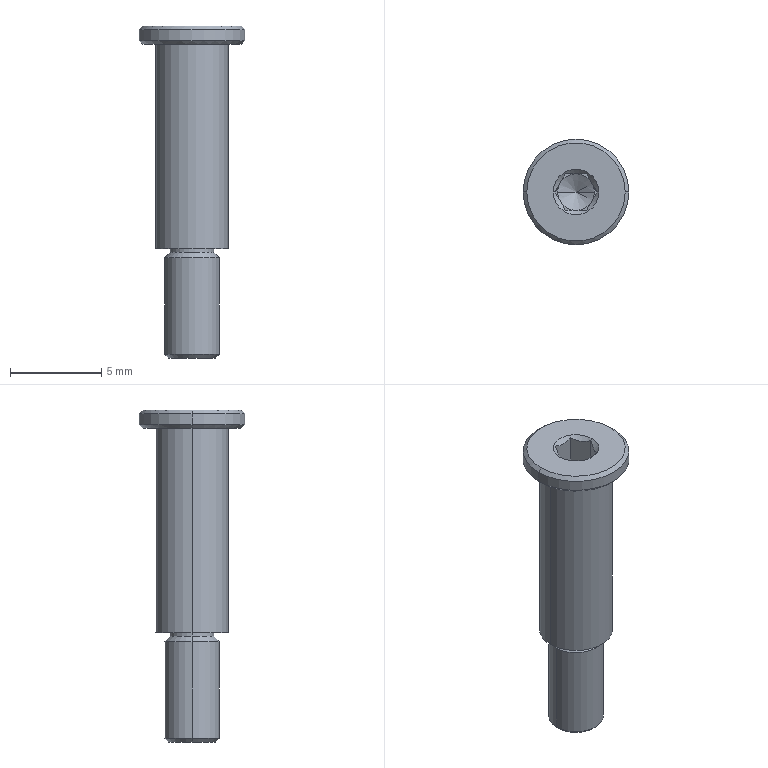Part | SolidWorks | features HoleWzd 1, ICE 1, Revolution 1 | 1 solid | 36 faces | box 5.8 x 5.8 x 18.2 mm | volume 198.341 mm3 | plane 16 | cone 12 | cylinder 8 | commonest cylinder face diameters 2.4 x2 3 x2 4 x2 5.8 x2
STEP:
#1=CARTESIAN_POINT('',(0.,0.,-3.101));
#2=VERTEX_POINT('',#1);
#3=CARTESIAN_POINT('',(1.,0.,-2.5));
#4=VERTEX_POINT('',#3);
#5=CARTESIAN_POINT('',(1.,0.,-2.5));
#6=DIRECTION('',(0.8572,0.,0.515));
#7=VECTOR('',#6,1000.);
#8=LINE('',#5,#7);
#9=EDGE_CURVE('',#2,#4,#8,.T.);
#10=ORIENTED_EDGE('',*,*,#9,.F.);
#11=CARTESIAN_POINT('',(-1.,0.,-2.5));
#12=VERTEX_POINT('',#11);
#13=CARTESIAN_POINT('',(-1.,0.,-2.5));
#14=DIRECTION('',(-0.8572,0.,0.515));
#15=VECTOR('',#14,1000.);
#16=LINE('',#13,#15);
#17=EDGE_CURVE('',#2,#12,#16,.T.);
#18=ORIENTED_EDGE('',*,*,#17,.T.);
#19=CARTESIAN_POINT('',(-0.866,-0.5,-2.5));
#20=VERTEX_POINT('',#19);
#21=CARTESIAN_POINT('',(0.,0.,-2.5));
#22=DIRECTION('',(0.,0.,1.));
#23=DIRECTION('',(1.,0.,0.));
#24=AXIS2_PLACEMENT_3D('',#21,#22,#23);
#25=CIRCLE('',#24,1.);
#26=EDGE_CURVE('',#12,#20,#25,.T.);
#27=ORIENTED_EDGE('',*,*,#26,.T.);
#28=CARTESIAN_POINT('',(0.,-1.,-2.5));
#29=VERTEX_POINT('',#28);
#30=CARTESIAN_POINT('',(0.,0.,-2.5));
#31=DIRECTION('',(0.,0.,1.));
#32=DIRECTION('',(1.,0.,0.));
#33=AXIS2_PLACEMENT_3D('',#30,#31,#32);
#34=CIRCLE('',#33,1.);
#35=EDGE_CURVE('',#20,#29,#34,.T.);
#36=ORIENTED_EDGE('',*,*,#35,.T.);
#37=CARTESIAN_POINT('',(0.866,-0.5,-2.5));
#38=VERTEX_POINT('',#37);
#39=CARTESIAN_POINT('',(0.,0.,-2.5));
#40=DIRECTION('',(0.,0.,1.));
#41=DIRECTION('',(1.,0.,0.));
#42=AXIS2_PLACEMENT_3D('',#39,#40,#41);
#43=CIRCLE('',#42,1.);
#44=EDGE_CURVE('',#29,#38,#43,.T.);
#45=ORIENTED_EDGE('',*,*,#44,.T.);
#46=CARTESIAN_POINT('',(0.,0.,-2.5));
#47=DIRECTION('',(0.,0.,1.));
#48=DIRECTION('',(1.,0.,0.));
#49=AXIS2_PLACEMENT_3D('',#46,#47,#48);
#50=CIRCLE('',#49,1.);
#51=EDGE_CURVE('',#38,#4,#50,.T.);
#52=ORIENTED_EDGE('',*,*,#51,.T.);
#53=EDGE_LOOP('',(#10,#18,#27,#36,#45,#52));
#54=FACE_OUTER_BOUND('',#53,.T.);
#55=CARTESIAN_POINT('',(0.,0.,-2.5));
#56=DIRECTION('',(0.,0.,1.));
#57=DIRECTION('',(1.,0.,0.));
#58=AXIS2_PLACEMENT_3D('',#55,#56,#57);
#59=CONICAL_SURFACE('',#58,1.,1.03);
#60=ADVANCED_FACE('',(#54),#59,.F.);
#61=CARTESIAN_POINT('',(-0.5774,-1.,-0.0953));
#62=VERTEX_POINT('',#61);
#63=CARTESIAN_POINT('',(-1.155,0.,-0.0953));
#64=VERTEX_POINT('',#63);
#65=CARTESIAN_POINT('',(-0.5774,-1.,-0.0953));
#66=CARTESIAN_POINT('',(-0.6225,-0.9219,-0.1404));
#67=CARTESIAN_POINT('',(-0.6686,-0.842,-0.1788));
#68=CARTESIAN_POINT('',(-0.7641,-0.6765,-0.2336));
#69=CARTESIAN_POINT('',(-0.8146,-0.5891,-0.2498));
#70=CARTESIAN_POINT('',(-0.9658,-0.3272,-0.2504));
#71=CARTESIAN_POINT('',(-1.064,-0.1572,-0.186));
#72=CARTESIAN_POINT('',(-1.155,0.,-0.0953));
#73=B_SPLINE_CURVE_WITH_KNOTS('',3,(#65,#66,#67,#68,#69,#70,#71,#72),.UNSPECIFIED.,.F.,.F.,(4,2,2,4),(0.000000254,0.0002984,0.0005966,0.001193),.UNSPECIFIED.);
#74=EDGE_CURVE('',#62,#64,#73,.T.);
#75=ORIENTED_EDGE('',*,*,#74,.T.);
#76=CARTESIAN_POINT('',(-1.25,0.,0.));
#77=VERTEX_POINT('',#76);
#78=CARTESIAN_POINT('',(-1.25,0.,0.));
#79=DIRECTION('',(-0.7071,0.,0.7071));
#80=VECTOR('',#79,1000.);
#81=LINE('',#78,#80);
#82=EDGE_CURVE('',#64,#77,#81,.T.);
#83=ORIENTED_EDGE('',*,*,#82,.T.);
#84=CARTESIAN_POINT('',(1.25,0.,0.));
#85=VERTEX_POINT('',#84);
#86=CARTESIAN_POINT('',(0.,0.,0.));
#87=DIRECTION('',(0.,0.,1.));
#88=DIRECTION('',(1.,0.,0.));
#89=AXIS2_PLACEMENT_3D('',#86,#87,#88);
#90=CIRCLE('',#89,1.25);
#91=EDGE_CURVE('',#77,#85,#90,.T.);
#92=ORIENTED_EDGE('',*,*,#91,.T.);
#93=CARTESIAN_POINT('',(1.155,0.,-0.0953));
#94=VERTEX_POINT('',#93);
#95=CARTESIAN_POINT('',(1.25,0.,0.));
#96=DIRECTION('',(0.7071,0.,0.7071));
#97=VECTOR('',#96,1000.);
#98=LINE('',#95,#97);
#99=EDGE_CURVE('',#94,#85,#98,.T.);
#100=ORIENTED_EDGE('',*,*,#99,.F.);
#101=CARTESIAN_POINT('',(0.5774,-1.,-0.0953));
#102=VERTEX_POINT('',#101);
#103=CARTESIAN_POINT('',(1.155,0.,-0.0953));
#104=CARTESIAN_POINT('',(1.11,-0.07813,-0.1404));
#105=CARTESIAN_POINT('',(1.063,-0.158,-0.1788));
#106=CARTESIAN_POINT('',(0.9679,-0.3235,-0.2336));
#107=CARTESIAN_POINT('',(0.9175,-0.4109,-0.2498));
#108=CARTESIAN_POINT('',(0.7663,-0.6728,-0.2504));
#109=CARTESIAN_POINT('',(0.6681,-0.8428,-0.186));
#110=CARTESIAN_POINT('',(0.5774,-1.,-0.0953));
#111=B_SPLINE_CURVE_WITH_KNOTS('',3,(#103,#104,#105,#106,#107,#108,#109,#110),.UNSPECIFIED.,.F.,.F.,(4,2,2,4),(0.000000254,0.0002984,0.0005966,0.001193),.UNSPECIFIED.);
#112=EDGE_CURVE('',#94,#102,#111,.T.);
#113=ORIENTED_EDGE('',*,*,#112,.T.);
#114=CARTESIAN_POINT('',(0.5774,-1.,-0.0953));
#115=CARTESIAN_POINT('',(0.3985,-1.,-0.1847));
#116=CARTESIAN_POINT('',(0.2033,-1.,-0.2499));
#117=CARTESIAN_POINT('',(-0.2019,-1.,-0.2501));
#118=CARTESIAN_POINT('',(-0.398,-1.,-0.185));
#119=CARTESIAN_POINT('',(-0.5774,-1.,-0.0953));
#120=B_SPLINE_CURVE_WITH_KNOTS('',3,(#114,#115,#116,#117,#118,#119),.UNSPECIFIED.,.F.,.F.,(4,2,4),(0.001472,0.002073,0.002675),.UNSPECIFIED.);
#121=EDGE_CURVE('',#102,#62,#120,.T.);
#122=ORIENTED_EDGE('',*,*,#121,.T.);
#123=EDGE_LOOP('',(#75,#83,#92,#100,#113,#122));
#124=FACE_OUTER_BOUND('',#123,.T.);
#125=CARTESIAN_POINT('',(0.,0.,0.));
#126=DIRECTION('',(0.,0.,1.));
#127=DIRECTION('',(1.,0.,0.));
#128=AXIS2_PLACEMENT_3D('',#125,#126,#127);
#129=CONICAL_SURFACE('',#128,1.25,0.7854);
#130=ADVANCED_FACE('',(#124),#129,.F.);
#131=CARTESIAN_POINT('',(1.3,0.,-18.2));
#132=VERTEX_POINT('',#131);
#133=CARTESIAN_POINT('',(-1.3,0.,-18.2));
#134=VERTEX_POINT('',#133);
#135=CARTESIAN_POINT('',(0.,0.,-18.2));
#136=DIRECTION('',(0.,0.,1.));
#137=DIRECTION('',(1.,0.,0.));
#138=AXIS2_PLACEMENT_3D('',#135,#136,#137);
#139=CIRCLE('',#138,1.3);
#140=EDGE_CURVE('',#132,#134,#139,.T.);
#141=ORIENTED_EDGE('',*,*,#140,.T.);
#142=CARTESIAN_POINT('',(-1.5,0.,-18.));
#143=VERTEX_POINT('',#142);
#144=CARTESIAN_POINT('',(-1.5,0.,-18.));
#145=DIRECTION('',(-0.7071,0.,0.7071));
#146=VECTOR('',#145,1000.);
#147=LINE('',#144,#146);
#148=EDGE_CURVE('',#134,#143,#147,.T.);
#149=ORIENTED_EDGE('',*,*,#148,.T.);
#150=CARTESIAN_POINT('',(1.5,0.,-18.));
#151=VERTEX_POINT('',#150);
#152=CARTESIAN_POINT('',(0.,0.,-18.));
#153=DIRECTION('',(0.,0.,1.));
#154=DIRECTION('',(1.,0.,0.));
#155=AXIS2_PLACEMENT_3D('',#152,#153,#154);
#156=CIRCLE('',#155,1.5);
#157=EDGE_CURVE('',#151,#143,#156,.T.);
#158=ORIENTED_EDGE('',*,*,#157,.F.);
#159=CARTESIAN_POINT('',(1.5,0.,-18.));
#160=DIRECTION('',(0.7071,0.,0.7071));
#161=VECTOR('',#160,1000.);
#162=LINE('',#159,#161);
#163=EDGE_CURVE('',#132,#151,#162,.T.);
#164=ORIENTED_EDGE('',*,*,#163,.F.);
#165=EDGE_LOOP('',(#141,#149,#158,#164));
#166=FACE_OUTER_BOUND('',#165,.T.);
#167=CARTESIAN_POINT('',(0.,0.,-18.));
#168=DIRECTION('',(0.,0.,1.));
#169=DIRECTION('',(1.,0.,0.));
#170=AXIS2_PLACEMENT_3D('',#167,#168,#169);
#171=CONICAL_SURFACE('',#170,1.5,0.7854);
#172=ADVANCED_FACE('',(#166),#171,.T.);
#173=ORIENTED_EDGE('',*,*,#157,.T.);
#174=CARTESIAN_POINT('',(-1.5,0.,-12.7));
#175=VERTEX_POINT('',#174);
#176=CARTESIAN_POINT('',(-1.5,0.,4.426));
#177=DIRECTION('',(0.,0.,1.));
#178=VECTOR('',#177,1000.);
#179=LINE('',#176,#178);
#180=EDGE_CURVE('',#143,#175,#179,.T.);
#181=ORIENTED_EDGE('',*,*,#180,.T.);
#182=CARTESIAN_POINT('',(1.5,0.,-12.7));
#183=VERTEX_POINT('',#182);
#184=CARTESIAN_POINT('',(0.,0.,-12.7));
#185=DIRECTION('',(0.,0.,1.));
#186=DIRECTION('',(1.,0.,0.));
#187=AXIS2_PLACEMENT_3D('',#184,#185,#186);
#188=CIRCLE('',#187,1.5);
#189=EDGE_CURVE('',#183,#175,#188,.T.);
#190=ORIENTED_EDGE('',*,*,#189,.F.);
#191=CARTESIAN_POINT('',(1.5,0.,4.426));
#192=DIRECTION('',(0.,0.,1.));
#193=VECTOR('',#192,1000.);
#194=LINE('',#191,#193);
#195=EDGE_CURVE('',#151,#183,#194,.T.);
#196=ORIENTED_EDGE('',*,*,#195,.F.);
#197=EDGE_LOOP('',(#173,#181,#190,#196));
#198=FACE_OUTER_BOUND('',#197,.T.);
#199=CARTESIAN_POINT('',(0.,0.,4.426));
#200=DIRECTION('',(0.,0.,1.));
#201=DIRECTION('',(1.,0.,0.));
#202=AXIS2_PLACEMENT_3D('',#199,#200,#201);
#203=CYLINDRICAL_SURFACE('',#202,1.5);
#204=ADVANCED_FACE('',(#198),#203,.T.);
#205=CARTESIAN_POINT('',(1.2,0.,-12.4));
#206=VERTEX_POINT('',#205);
#207=CARTESIAN_POINT('',(-1.2,0.,-12.4));
#208=VERTEX_POINT('',#207);
#209=CARTESIAN_POINT('',(0.,0.,-12.4));
#210=DIRECTION('',(0.,0.,1.));
#211=DIRECTION('',(1.,0.,0.));
#212=AXIS2_PLACEMENT_3D('',#209,#210,#211);
#213=CIRCLE('',#212,1.2);
#214=EDGE_CURVE('',#206,#208,#213,.T.);
#215=ORIENTED_EDGE('',*,*,#214,.F.);
#216=CARTESIAN_POINT('',(1.2,0.,-12.4));
#217=DIRECTION('',(0.7071,0.,-0.7071));
#218=VECTOR('',#217,1000.);
#219=LINE('',#216,#218);
#220=EDGE_CURVE('',#206,#183,#219,.T.);
#221=ORIENTED_EDGE('',*,*,#220,.T.);
#222=ORIENTED_EDGE('',*,*,#189,.T.);
#223=CARTESIAN_POINT('',(-1.2,0.,-12.4));
#224=DIRECTION('',(-0.7071,0.,-0.7071));
#225=VECTOR('',#224,1000.);
#226=LINE('',#223,#225);
#227=EDGE_CURVE('',#208,#175,#226,.T.);
#228=ORIENTED_EDGE('',*,*,#227,.F.);
#229=EDGE_LOOP('',(#215,#221,#222,#228));
#230=FACE_OUTER_BOUND('',#229,.T.);
#231=CARTESIAN_POINT('',(0.,0.,-12.4));
#232=DIRECTION('',(0.,0.,-1.));
#233=DIRECTION('',(-1.,0.,0.));
#234=AXIS2_PLACEMENT_3D('',#231,#232,#233);
#235=CONICAL_SURFACE('',#234,1.2,0.7854);
#236=ADVANCED_FACE('',(#230),#235,.T.);
#237=ORIENTED_EDGE('',*,*,#214,.T.);
#238=CARTESIAN_POINT('',(-1.2,0.,-12.2));
#239=VERTEX_POINT('',#238);
#240=CARTESIAN_POINT('',(-1.2,0.,4.426));
#241=DIRECTION('',(0.,0.,1.));
#242=VECTOR('',#241,1000.);
#243=LINE('',#240,#242);
#244=EDGE_CURVE('',#208,#239,#243,.T.);
#245=ORIENTED_EDGE('',*,*,#244,.T.);
#246=CARTESIAN_POINT('',(1.2,0.,-12.2));
#247=VERTEX_POINT('',#246);
#248=CARTESIAN_POINT('',(0.,0.,-12.2));
#249=DIRECTION('',(0.,0.,1.));
#250=DIRECTION('',(1.,0.,0.));
#251=AXIS2_PLACEMENT_3D('',#248,#249,#250);
#252=CIRCLE('',#251,1.2);
#253=EDGE_CURVE('',#247,#239,#252,.T.);
#254=ORIENTED_EDGE('',*,*,#253,.F.);
#255=CARTESIAN_POINT('',(1.2,0.,4.426));
#256=DIRECTION('',(0.,0.,1.));
#257=VECTOR('',#256,1000.);
#258=LINE('',#255,#257);
#259=EDGE_CURVE('',#206,#247,#258,.T.);
#260=ORIENTED_EDGE('',*,*,#259,.F.);
#261=EDGE_LOOP('',(#237,#245,#254,#260));
#262=FACE_OUTER_BOUND('',#261,.T.);
#263=CARTESIAN_POINT('',(0.,0.,4.426));
#264=DIRECTION('',(0.,0.,1.));
#265=DIRECTION('',(1.,0.,0.));
#266=AXIS2_PLACEMENT_3D('',#263,#264,#265);
#267=CYLINDRICAL_SURFACE('',#266,1.2);
#268=ADVANCED_FACE('',(#262),#267,.T.);
#269=CARTESIAN_POINT('',(2.,0.,-12.2));
#270=VERTEX_POINT('',#269);
#271=CARTESIAN_POINT('',(-2.,0.,-12.2));
#272=VERTEX_POINT('',#271);
#273=CARTESIAN_POINT('',(0.,0.,-12.2));
#274=DIRECTION('',(0.,0.,1.));
#275=DIRECTION('',(1.,0.,0.));
#276=AXIS2_PLACEMENT_3D('',#273,#274,#275);
#277=CIRCLE('',#276,2.);
#278=EDGE_CURVE('',#270,#272,#277,.T.);
#279=ORIENTED_EDGE('',*,*,#278,.T.);
#280=CARTESIAN_POINT('',(-2.,0.,-1.));
#281=VERTEX_POINT('',#280);
#282=CARTESIAN_POINT('',(-2.,0.,4.426));
#283=DIRECTION('',(0.,0.,1.));
#284=VECTOR('',#283,1000.);
#285=LINE('',#282,#284);
#286=EDGE_CURVE('',#272,#281,#285,.T.);
#287=ORIENTED_EDGE('',*,*,#286,.T.);
#288=CARTESIAN_POINT('',(2.,0.,-1.));
#289=VERTEX_POINT('',#288);
#290=CARTESIAN_POINT('',(0.,0.,-1.));
#291=DIRECTION('',(0.,0.,1.));
#292=DIRECTION('',(1.,0.,0.));
#293=AXIS2_PLACEMENT_3D('',#290,#291,#292);
#294=CIRCLE('',#293,2.);
#295=EDGE_CURVE('',#289,#281,#294,.T.);
#296=ORIENTED_EDGE('',*,*,#295,.F.);
#297=CARTESIAN_POINT('',(2.,0.,4.426));
#298=DIRECTION('',(0.,0.,1.));
#299=VECTOR('',#298,1000.);
#300=LINE('',#297,#299);
#301=EDGE_CURVE('',#270,#289,#300,.T.);
#302=ORIENTED_EDGE('',*,*,#301,.F.);
#303=EDGE_LOOP('',(#279,#287,#296,#302));
#304=FACE_OUTER_BOUND('',#303,.T.);
#305=CARTESIAN_POINT('',(0.,0.,4.426));
#306=DIRECTION('',(0.,0.,1.));
#307=DIRECTION('',(1.,0.,0.));
#308=AXIS2_PLACEMENT_3D('',#305,#306,#307);
#309=CYLINDRICAL_SURFACE('',#308,2.);
#310=ADVANCED_FACE('',(#304),#309,.T.);
#311=CARTESIAN_POINT('',(2.7,0.,-1.));
#312=VERTEX_POINT('',#311);
#313=CARTESIAN_POINT('',(-2.7,0.,-1.));
#314=VERTEX_POINT('',#313);
#315=CARTESIAN_POINT('',(0.,0.,-1.));
#316=DIRECTION('',(0.,0.,1.));
#317=DIRECTION('',(1.,0.,0.));
#318=AXIS2_PLACEMENT_3D('',#315,#316,#317);
#319=CIRCLE('',#318,2.7);
#320=EDGE_CURVE('',#312,#314,#319,.T.);
#321=ORIENTED_EDGE('',*,*,#320,.T.);
#322=CARTESIAN_POINT('',(-2.9,0.,-0.8));
#323=VERTEX_POINT('',#322);
#324=CARTESIAN_POINT('',(-2.9,0.,-0.8));
#325=DIRECTION('',(-0.7071,0.,0.7071));
#326=VECTOR('',#325,1000.);
#327=LINE('',#324,#326);
#328=EDGE_CURVE('',#314,#323,#327,.T.);
#329=ORIENTED_EDGE('',*,*,#328,.T.);
#330=CARTESIAN_POINT('',(2.9,0.,-0.8));
#331=VERTEX_POINT('',#330);
#332=CARTESIAN_POINT('',(0.,0.,-0.8));
#333=DIRECTION('',(0.,0.,1.));
#334=DIRECTION('',(1.,0.,0.));
#335=AXIS2_PLACEMENT_3D('',#332,#333,#334);
#336=CIRCLE('',#335,2.9);
#337=EDGE_CURVE('',#331,#323,#336,.T.);
#338=ORIENTED_EDGE('',*,*,#337,.F.);
#339=CARTESIAN_POINT('',(2.9,0.,-0.8));
#340=DIRECTION('',(0.7071,0.,0.7071));
#341=VECTOR('',#340,1000.);
#342=LINE('',#339,#341);
#343=EDGE_CURVE('',#312,#331,#342,.T.);
#344=ORIENTED_EDGE('',*,*,#343,.F.);
#345=EDGE_LOOP('',(#321,#329,#338,#344));
#346=FACE_OUTER_BOUND('',#345,.T.);
#347=CARTESIAN_POINT('',(0.,0.,-0.8));
#348=DIRECTION('',(0.,0.,1.));
#349=DIRECTION('',(1.,0.,0.));
#350=AXIS2_PLACEMENT_3D('',#347,#348,#349);
#351=CONICAL_SURFACE('',#350,2.9,0.7854);
#352=ADVANCED_FACE('',(#346),#351,.T.);
#353=ORIENTED_EDGE('',*,*,#337,.T.);
#354=CARTESIAN_POINT('',(-2.9,0.,-0.2));
#355=VERTEX_POINT('',#354);
#356=CARTESIAN_POINT('',(-2.9,0.,4.426));
#357=DIRECTION('',(0.,0.,1.));
#358=VECTOR('',#357,1000.);
#359=LINE('',#356,#358);
#360=EDGE_CURVE('',#323,#355,#359,.T.);
#361=ORIENTED_EDGE('',*,*,#360,.T.);
#362=CARTESIAN_POINT('',(2.9,0.,-0.2));
#363=VERTEX_POINT('',#362);
#364=CARTESIAN_POINT('',(0.,0.,-0.2));
#365=DIRECTION('',(0.,0.,1.));
#366=DIRECTION('',(1.,0.,0.));
#367=AXIS2_PLACEMENT_3D('',#364,#365,#366);
#368=CIRCLE('',#367,2.9);
#369=EDGE_CURVE('',#363,#355,#368,.T.);
#370=ORIENTED_EDGE('',*,*,#369,.F.);
#371=CARTESIAN_POINT('',(2.9,0.,4.426));
#372=DIRECTION('',(0.,0.,1.));
#373=VECTOR('',#372,1000.);
#374=LINE('',#371,#373);
#375=EDGE_CURVE('',#331,#363,#374,.T.);
#376=ORIENTED_EDGE('',*,*,#375,.F.);
#377=EDGE_LOOP('',(#353,#361,#370,#376));
#378=FACE_OUTER_BOUND('',#377,.T.);
#379=CARTESIAN_POINT('',(0.,0.,4.426));
#380=DIRECTION('',(0.,0.,1.));
#381=DIRECTION('',(1.,0.,0.));
#382=AXIS2_PLACEMENT_3D('',#379,#380,#381);
#383=CYLINDRICAL_SURFACE('',#382,2.9);
#384=ADVANCED_FACE('',(#378),#383,.T.);
#385=CARTESIAN_POINT('',(2.7,0.,0.));
#386=VERTEX_POINT('',#385);
#387=CARTESIAN_POINT('',(-2.7,0.,0.));
#388=VERTEX_POINT('',#387);
#389=CARTESIAN_POINT('',(0.,0.,0.));
#390=DIRECTION('',(0.,0.,1.));
#391=DIRECTION('',(1.,0.,0.));
#392=AXIS2_PLACEMENT_3D('',#389,#390,#391);
#393=CIRCLE('',#392,2.7);
#394=EDGE_CURVE('',#386,#388,#393,.T.);
#395=ORIENTED_EDGE('',*,*,#394,.F.);
#396=CARTESIAN_POINT('',(2.7,0.,0.));
#397=DIRECTION('',(0.7071,0.,-0.7071));
#398=VECTOR('',#397,1000.);
#399=LINE('',#396,#398);
#400=EDGE_CURVE('',#386,#363,#399,.T.);
#401=ORIENTED_EDGE('',*,*,#400,.T.);
#402=ORIENTED_EDGE('',*,*,#369,.T.);
#403=CARTESIAN_POINT('',(-2.7,0.,0.));
#404=DIRECTION('',(-0.7071,0.,-0.7071));
#405=VECTOR('',#404,1000.);
#406=LINE('',#403,#405);
#407=EDGE_CURVE('',#388,#355,#406,.T.);
#408=ORIENTED_EDGE('',*,*,#407,.F.);
#409=EDGE_LOOP('',(#395,#401,#402,#408));
#410=FACE_OUTER_BOUND('',#409,.T.);
#411=CARTESIAN_POINT('',(0.,0.,0.));
#412=DIRECTION('',(0.,0.,-1.));
#413=DIRECTION('',(-1.,0.,0.));
#414=AXIS2_PLACEMENT_3D('',#411,#412,#413);
#415=CONICAL_SURFACE('',#414,2.7,0.7854);
#416=ADVANCED_FACE('',(#410),#415,.T.);
#417=CARTESIAN_POINT('',(0.,0.,0.));
#418=DIRECTION('',(0.,0.,1.));
#419=DIRECTION('',(1.,0.,0.));
#420=AXIS2_PLACEMENT_3D('',#417,#418,#419);
#421=CIRCLE('',#420,1.25);
#422=EDGE_CURVE('',#85,#77,#421,.T.);
#423=ORIENTED_EDGE('',*,*,#422,.F.);
#424=ORIENTED_EDGE('',*,*,#91,.F.);
#425=EDGE_LOOP('',(#423,#424));
#426=FACE_BOUND('',#425,.T.);
#427=CARTESIAN_POINT('',(0.,0.,0.));
#428=DIRECTION('',(0.,0.,1.));
#429=DIRECTION('',(1.,0.,0.));
#430=AXIS2_PLACEMENT_3D('',#427,#428,#429);
#431=CIRCLE('',#430,2.7);
#432=EDGE_CURVE('',#388,#386,#431,.T.);
#433=ORIENTED_EDGE('',*,*,#432,.T.);
#434=ORIENTED_EDGE('',*,*,#394,.T.);
#435=EDGE_LOOP('',(#433,#434));
#436=FACE_OUTER_BOUND('',#435,.T.);
#437=CARTESIAN_POINT('',(0.,0.,0.));
#438=DIRECTION('',(0.,0.,1.));
#439=DIRECTION('',(1.,0.,0.));
#440=AXIS2_PLACEMENT_3D('',#437,#438,#439);
#441=PLANE('',#440);
#442=ADVANCED_FACE('',(#426,#436),#441,.T.);
#443=ORIENTED_EDGE('',*,*,#400,.F.);
#444=ORIENTED_EDGE('',*,*,#432,.F.);
#445=ORIENTED_EDGE('',*,*,#407,.T.);
#446=CARTESIAN_POINT('',(0.,0.,-0.2));
#447=DIRECTION('',(0.,0.,1.));
#448=DIRECTION('',(1.,0.,0.));
#449=AXIS2_PLACEMENT_3D('',#446,#447,#448);
#450=CIRCLE('',#449,2.9);
#451=EDGE_CURVE('',#355,#363,#450,.T.);
#452=ORIENTED_EDGE('',*,*,#451,.T.);
#453=EDGE_LOOP('',(#443,#444,#445,#452));
#454=FACE_OUTER_BOUND('',#453,.T.);
#455=CARTESIAN_POINT('',(0.,0.,0.));
#456=DIRECTION('',(0.,0.,-1.));
#457=DIRECTION('',(-1.,0.,0.));
#458=AXIS2_PLACEMENT_3D('',#455,#456,#457);
#459=CONICAL_SURFACE('',#458,2.7,0.7854);
#460=ADVANCED_FACE('',(#454),#459,.T.);
#461=ORIENTED_EDGE('',*,*,#360,.F.);
#462=CARTESIAN_POINT('',(0.,0.,-0.8));
#463=DIRECTION('',(0.,0.,1.));
#464=DIRECTION('',(1.,0.,0.));
#465=AXIS2_PLACEMENT_3D('',#462,#463,#464);
#466=CIRCLE('',#465,2.9);
#467=EDGE_CURVE('',#323,#331,#466,.T.);
#468=ORIENTED_EDGE('',*,*,#467,.T.);
#469=ORIENTED_EDGE('',*,*,#375,.T.);
#470=ORIENTED_EDGE('',*,*,#451,.F.);
#471=EDGE_LOOP('',(#461,#468,#469,#470));
#472=FACE_OUTER_BOUND('',#471,.T.);
#473=CARTESIAN_POINT('',(0.,0.,4.426));
#474=DIRECTION('',(0.,0.,1.));
#475=DIRECTION('',(1.,0.,0.));
#476=AXIS2_PLACEMENT_3D('',#473,#474,#475);
#477=CYLINDRICAL_SURFACE('',#476,2.9);
#478=ADVANCED_FACE('',(#472),#477,.T.);
#479=ORIENTED_EDGE('',*,*,#328,.F.);
#480=CARTESIAN_POINT('',(0.,0.,-1.));
#481=DIRECTION('',(0.,0.,1.));
#482=DIRECTION('',(1.,0.,0.));
#483=AXIS2_PLACEMENT_3D('',#480,#481,#482);
#484=CIRCLE('',#483,2.7);
#485=EDGE_CURVE('',#314,#312,#484,.T.);
#486=ORIENTED_EDGE('',*,*,#485,.T.);
#487=ORIENTED_EDGE('',*,*,#343,.T.);
#488=ORIENTED_EDGE('',*,*,#467,.F.);
#489=EDGE_LOOP('',(#479,#486,#487,#488));
#490=FACE_OUTER_BOUND('',#489,.T.);
#491=CARTESIAN_POINT('',(0.,0.,-0.8));
#492=DIRECTION('',(0.,0.,1.));
#493=DIRECTION('',(1.,0.,0.));
#494=AXIS2_PLACEMENT_3D('',#491,#492,#493);
#495=CONICAL_SURFACE('',#494,2.9,0.7854);
#496=ADVANCED_FACE('',(#490),#495,.T.);
#497=ORIENTED_EDGE('',*,*,#295,.T.);
#498=CARTESIAN_POINT('',(0.,0.,-1.));
#499=DIRECTION('',(0.,0.,1.));
#500=DIRECTION('',(1.,0.,0.));
#501=AXIS2_PLACEMENT_3D('',#498,#499,#500);
#502=CIRCLE('',#501,2.);
#503=EDGE_CURVE('',#281,#289,#502,.T.);
#504=ORIENTED_EDGE('',*,*,#503,.T.);
#505=EDGE_LOOP('',(#497,#504));
#506=FACE_BOUND('',#505,.T.);
#507=ORIENTED_EDGE('',*,*,#320,.F.);
#508=ORIENTED_EDGE('',*,*,#485,.F.);
#509=EDGE_LOOP('',(#507,#508));
#510=FACE_OUTER_BOUND('',#509,.T.);
#511=CARTESIAN_POINT('',(2.7,0.,-1.));
#512=DIRECTION('',(0.,0.,-1.));
#513=DIRECTION('',(-1.,0.,0.));
#514=AXIS2_PLACEMENT_3D('',#511,#512,#513);
#515=PLANE('',#514);
#516=ADVANCED_FACE('',(#506,#510),#515,.T.);
#517=ORIENTED_EDGE('',*,*,#286,.F.);
#518=CARTESIAN_POINT('',(0.,0.,-12.2));
#519=DIRECTION('',(0.,0.,1.));
#520=DIRECTION('',(1.,0.,0.));
#521=AXIS2_PLACEMENT_3D('',#518,#519,#520);
#522=CIRCLE('',#521,2.);
#523=EDGE_CURVE('',#272,#270,#522,.T.);
#524=ORIENTED_EDGE('',*,*,#523,.T.);
#525=ORIENTED_EDGE('',*,*,#301,.T.);
#526=ORIENTED_EDGE('',*,*,#503,.F.);
#527=EDGE_LOOP('',(#517,#524,#525,#526));
#528=FACE_OUTER_BOUND('',#527,.T.);
#529=CARTESIAN_POINT('',(0.,0.,4.426));
#530=DIRECTION('',(0.,0.,1.));
#531=DIRECTION('',(1.,0.,0.));
#532=AXIS2_PLACEMENT_3D('',#529,#530,#531);
#533=CYLINDRICAL_SURFACE('',#532,2.);
#534=ADVANCED_FACE('',(#528),#533,.T.);
#535=ORIENTED_EDGE('',*,*,#253,.T.);
#536=CARTESIAN_POINT('',(0.,0.,-12.2));
#537=DIRECTION('',(0.,0.,1.));
#538=DIRECTION('',(1.,0.,0.));
#539=AXIS2_PLACEMENT_3D('',#536,#537,#538);
#540=CIRCLE('',#539,1.2);
#541=EDGE_CURVE('',#239,#247,#540,.T.);
#542=ORIENTED_EDGE('',*,*,#541,.T.);
#543=EDGE_LOOP('',(#535,#542));
#544=FACE_BOUND('',#543,.T.);
#545=ORIENTED_EDGE('',*,*,#278,.F.);
#546=ORIENTED_EDGE('',*,*,#523,.F.);
#547=EDGE_LOOP('',(#545,#546));
#548=FACE_OUTER_BOUND('',#547,.T.);
#549=CARTESIAN_POINT('',(2.,0.,-12.2));
#550=DIRECTION('',(0.,0.,-1.));
#551=DIRECTION('',(-1.,0.,0.));
#552=AXIS2_PLACEMENT_3D('',#549,#550,#551);
#553=PLANE('',#552);
#554=ADVANCED_FACE('',(#544,#548),#553,.T.);
#555=ORIENTED_EDGE('',*,*,#244,.F.);
#556=CARTESIAN_POINT('',(0.,0.,-12.4));
#557=DIRECTION('',(0.,0.,1.));
#558=DIRECTION('',(1.,0.,0.));
#559=AXIS2_PLACEMENT_3D('',#556,#557,#558);
#560=CIRCLE('',#559,1.2);
#561=EDGE_CURVE('',#208,#206,#560,.T.);
#562=ORIENTED_EDGE('',*,*,#561,.T.);
#563=ORIENTED_EDGE('',*,*,#259,.T.);
#564=ORIENTED_EDGE('',*,*,#541,.F.);
#565=EDGE_LOOP('',(#555,#562,#563,#564));
#566=FACE_OUTER_BOUND('',#565,.T.);
#567=CARTESIAN_POINT('',(0.,0.,4.426));
#568=DIRECTION('',(0.,0.,1.));
#569=DIRECTION('',(1.,0.,0.));
#570=AXIS2_PLACEMENT_3D('',#567,#568,#569);
#571=CYLINDRICAL_SURFACE('',#570,1.2);
#572=ADVANCED_FACE('',(#566),#571,.T.);
#573=ORIENTED_EDGE('',*,*,#220,.F.);
#574=ORIENTED_EDGE('',*,*,#561,.F.);
#575=ORIENTED_EDGE('',*,*,#227,.T.);
#576=CARTESIAN_POINT('',(0.,0.,-12.7));
#577=DIRECTION('',(0.,0.,1.));
#578=DIRECTION('',(1.,0.,0.));
#579=AXIS2_PLACEMENT_3D('',#576,#577,#578);
#580=CIRCLE('',#579,1.5);
#581=EDGE_CURVE('',#175,#183,#580,.T.);
#582=ORIENTED_EDGE('',*,*,#581,.T.);
#583=EDGE_LOOP('',(#573,#574,#575,#582));
#584=FACE_OUTER_BOUND('',#583,.T.);
#585=CARTESIAN_POINT('',(0.,0.,-12.4));
#586=DIRECTION('',(0.,0.,-1.));
#587=DIRECTION('',(-1.,0.,0.));
#588=AXIS2_PLACEMENT_3D('',#585,#586,#587);
#589=CONICAL_SURFACE('',#588,1.2,0.7854);
#590=ADVANCED_FACE('',(#584),#589,.T.);
#591=ORIENTED_EDGE('',*,*,#180,.F.);
#592=CARTESIAN_POINT('',(0.,0.,-18.));
#593=DIRECTION('',(0.,0.,1.));
#594=DIRECTION('',(1.,0.,0.));
#595=AXIS2_PLACEMENT_3D('',#592,#593,#594);
#596=CIRCLE('',#595,1.5);
#597=EDGE_CURVE('',#143,#151,#596,.T.);
#598=ORIENTED_EDGE('',*,*,#597,.T.);
#599=ORIENTED_EDGE('',*,*,#195,.T.);
#600=ORIENTED_EDGE('',*,*,#581,.F.);
#601=EDGE_LOOP('',(#591,#598,#599,#600));
#602=FACE_OUTER_BOUND('',#601,.T.);
#603=CARTESIAN_POINT('',(0.,0.,4.426));
#604=DIRECTION('',(0.,0.,1.));
#605=DIRECTION('',(1.,0.,0.));
#606=AXIS2_PLACEMENT_3D('',#603,#604,#605);
#607=CYLINDRICAL_SURFACE('',#606,1.5);
#608=ADVANCED_FACE('',(#602),#607,.T.);
#609=ORIENTED_EDGE('',*,*,#148,.F.);
#610=CARTESIAN_POINT('',(0.,0.,-18.2));
#611=DIRECTION('',(0.,0.,1.));
#612=DIRECTION('',(1.,0.,0.));
#613=AXIS2_PLACEMENT_3D('',#610,#611,#612);
#614=CIRCLE('',#613,1.3);
#615=EDGE_CURVE('',#134,#132,#614,.T.);
#616=ORIENTED_EDGE('',*,*,#615,.T.);
#617=ORIENTED_EDGE('',*,*,#163,.T.);
#618=ORIENTED_EDGE('',*,*,#597,.F.);
#619=EDGE_LOOP('',(#609,#616,#617,#618));
#620=FACE_OUTER_BOUND('',#619,.T.);
#621=CARTESIAN_POINT('',(0.,0.,-18.));
#622=DIRECTION('',(0.,0.,1.));
#623=DIRECTION('',(1.,0.,0.));
#624=AXIS2_PLACEMENT_3D('',#621,#622,#623);
#625=CONICAL_SURFACE('',#624,1.5,0.7854);
#626=ADVANCED_FACE('',(#620),#625,.T.);
#627=ORIENTED_EDGE('',*,*,#140,.F.);
#628=ORIENTED_EDGE('',*,*,#615,.F.);
#629=EDGE_LOOP('',(#627,#628));
#630=FACE_OUTER_BOUND('',#629,.T.);
#631=CARTESIAN_POINT('',(1.3,0.,-18.2));
#632=DIRECTION('',(0.,0.,-1.));
#633=DIRECTION('',(-1.,0.,0.));
#634=AXIS2_PLACEMENT_3D('',#631,#632,#633);
#635=PLANE('',#634);
#636=ADVANCED_FACE('',(#630),#635,.T.);
#637=ORIENTED_EDGE('',*,*,#82,.F.);
#638=CARTESIAN_POINT('',(-0.5774,1.,-0.0953));
#639=VERTEX_POINT('',#638);
#640=CARTESIAN_POINT('',(-1.155,0.,-0.0953));
#641=CARTESIAN_POINT('',(-1.11,0.07813,-0.1404));
#642=CARTESIAN_POINT('',(-1.063,0.158,-0.1788));
#643=CARTESIAN_POINT('',(-0.9679,0.3235,-0.2336));
#644=CARTESIAN_POINT('',(-0.9175,0.4109,-0.2498));
#645=CARTESIAN_POINT('',(-0.7663,0.6728,-0.2504));
#646=CARTESIAN_POINT('',(-0.6681,0.8428,-0.186));
#647=CARTESIAN_POINT('',(-0.5774,1.,-0.0953));
#648=B_SPLINE_CURVE_WITH_KNOTS('',3,(#640,#641,#642,#643,#644,#645,#646,#647),.UNSPECIFIED.,.F.,.F.,(4,2,2,4),(0.000000254,0.0002984,0.0005966,0.001193),.UNSPECIFIED.);
#649=EDGE_CURVE('',#64,#639,#648,.T.);
#650=ORIENTED_EDGE('',*,*,#649,.T.);
#651=CARTESIAN_POINT('',(0.5774,1.,-0.0953));
#652=VERTEX_POINT('',#651);
#653=CARTESIAN_POINT('',(-0.5774,1.,-0.0953));
#654=CARTESIAN_POINT('',(-0.3985,1.,-0.1847));
#655=CARTESIAN_POINT('',(-0.2033,1.,-0.2499));
#656=CARTESIAN_POINT('',(0.2019,1.,-0.2501));
#657=CARTESIAN_POINT('',(0.398,1.,-0.185));
#658=CARTESIAN_POINT('',(0.5774,1.,-0.0953));
#659=B_SPLINE_CURVE_WITH_KNOTS('',3,(#653,#654,#655,#656,#657,#658),.UNSPECIFIED.,.F.,.F.,(4,2,4),(0.001472,0.002073,0.002675),.UNSPECIFIED.);
#660=EDGE_CURVE('',#639,#652,#659,.T.);
#661=ORIENTED_EDGE('',*,*,#660,.T.);
#662=CARTESIAN_POINT('',(0.5774,1.,-0.0953));
#663=CARTESIAN_POINT('',(0.6225,0.9219,-0.1404));
#664=CARTESIAN_POINT('',(0.6686,0.842,-0.1788));
#665=CARTESIAN_POINT('',(0.7641,0.6765,-0.2336));
#666=CARTESIAN_POINT('',(0.8146,0.5891,-0.2498));
#667=CARTESIAN_POINT('',(0.9658,0.3272,-0.2504));
#668=CARTESIAN_POINT('',(1.064,0.1572,-0.186));
#669=CARTESIAN_POINT('',(1.155,0.,-0.0953));
#670=B_SPLINE_CURVE_WITH_KNOTS('',3,(#662,#663,#664,#665,#666,#667,#668,#669),.UNSPECIFIED.,.F.,.F.,(4,2,2,4),(0.000000254,0.0002984,0.0005966,0.001193),.UNSPECIFIED.);
#671=EDGE_CURVE('',#652,#94,#670,.T.);
#672=ORIENTED_EDGE('',*,*,#671,.T.);
#673=ORIENTED_EDGE('',*,*,#99,.T.);
#674=ORIENTED_EDGE('',*,*,#422,.T.);
#675=EDGE_LOOP('',(#637,#650,#661,#672,#673,#674));
#676=FACE_OUTER_BOUND('',#675,.T.);
#677=CARTESIAN_POINT('',(0.,0.,0.));
#678=DIRECTION('',(0.,0.,1.));
#679=DIRECTION('',(1.,0.,0.));
#680=AXIS2_PLACEMENT_3D('',#677,#678,#679);
#681=CONICAL_SURFACE('',#680,1.25,0.7854);
#682=ADVANCED_FACE('',(#676),#681,.F.);
#683=ORIENTED_EDGE('',*,*,#44,.F.);
#684=CARTESIAN_POINT('',(0.5774,-1.,-2.5));
#685=VERTEX_POINT('',#684);
#686=CARTESIAN_POINT('',(-0.5774,-1.,-2.5));
#687=DIRECTION('',(1.,0.,0.));
#688=VECTOR('',#687,1000.);
#689=LINE('',#686,#688);
#690=EDGE_CURVE('',#29,#685,#689,.T.);
#691=ORIENTED_EDGE('',*,*,#690,.T.);
#692=CARTESIAN_POINT('',(0.5774,-1.,-2.5));
#693=DIRECTION('',(0.5,0.866,0.));
#694=VECTOR('',#693,1000.);
#695=LINE('',#692,#694);
#696=EDGE_CURVE('',#685,#38,#695,.T.);
#697=ORIENTED_EDGE('',*,*,#696,.T.);
#698=EDGE_LOOP('',(#683,#691,#697));
#699=FACE_OUTER_BOUND('',#698,.T.);
#700=CARTESIAN_POINT('',(0.,0.,-2.5));
#701=DIRECTION('',(0.,0.,1.));
#702=DIRECTION('',(1.,0.,0.));
#703=AXIS2_PLACEMENT_3D('',#700,#701,#702);
#704=PLANE('',#703);
#705=ADVANCED_FACE('',(#699),#704,.T.);
#706=ORIENTED_EDGE('',*,*,#35,.F.);
#707=CARTESIAN_POINT('',(-0.5774,-1.,-2.5));
#708=VERTEX_POINT('',#707);
#709=CARTESIAN_POINT('',(-1.155,0.,-2.5));
#710=DIRECTION('',(0.5,-0.866,0.));
#711=VECTOR('',#710,1000.);
#712=LINE('',#709,#711);
#713=EDGE_CURVE('',#20,#708,#712,.T.);
#714=ORIENTED_EDGE('',*,*,#713,.T.);
#715=CARTESIAN_POINT('',(-0.5774,-1.,-2.5));
#716=DIRECTION('',(1.,0.,0.));
#717=VECTOR('',#716,1000.);
#718=LINE('',#715,#717);
#719=EDGE_CURVE('',#708,#29,#718,.T.);
#720=ORIENTED_EDGE('',*,*,#719,.T.);
#721=EDGE_LOOP('',(#706,#714,#720));
#722=FACE_OUTER_BOUND('',#721,.T.);
#723=CARTESIAN_POINT('',(0.,0.,-2.5));
#724=DIRECTION('',(0.,0.,1.));
#725=DIRECTION('',(1.,0.,0.));
#726=AXIS2_PLACEMENT_3D('',#723,#724,#725);
#727=PLANE('',#726);
#728=ADVANCED_FACE('',(#722),#727,.T.);
#729=CARTESIAN_POINT('',(-0.866,0.5,-2.5));
#730=VERTEX_POINT('',#729);
#731=CARTESIAN_POINT('',(0.,0.,-2.5));
#732=DIRECTION('',(0.,0.,1.));
#733=DIRECTION('',(1.,0.,0.));
#734=AXIS2_PLACEMENT_3D('',#731,#732,#733);
#735=CIRCLE('',#734,1.);
#736=EDGE_CURVE('',#730,#12,#735,.T.);
#737=ORIENTED_EDGE('',*,*,#736,.F.);
#738=CARTESIAN_POINT('',(-1.155,0.,-2.5));
#739=VERTEX_POINT('',#738);
#740=CARTESIAN_POINT('',(-0.5774,1.,-2.5));
#741=DIRECTION('',(-0.5,-0.866,0.));
#742=VECTOR('',#741,1000.);
#743=LINE('',#740,#742);
#744=EDGE_CURVE('',#730,#739,#743,.T.);
#745=ORIENTED_EDGE('',*,*,#744,.T.);
#746=CARTESIAN_POINT('',(-1.155,0.,-2.5));
#747=DIRECTION('',(0.5,-0.866,0.));
#748=VECTOR('',#747,1000.);
#749=LINE('',#746,#748);
#750=EDGE_CURVE('',#739,#20,#749,.T.);
#751=ORIENTED_EDGE('',*,*,#750,.T.);
#752=ORIENTED_EDGE('',*,*,#26,.F.);
#753=EDGE_LOOP('',(#737,#745,#751,#752));
#754=FACE_OUTER_BOUND('',#753,.T.);
#755=CARTESIAN_POINT('',(0.,0.,-2.5));
#756=DIRECTION('',(0.,0.,1.));
#757=DIRECTION('',(1.,0.,0.));
#758=AXIS2_PLACEMENT_3D('',#755,#756,#757);
#759=PLANE('',#758);
#760=ADVANCED_FACE('',(#754),#759,.T.);
#761=CARTESIAN_POINT('',(0.,1.,-2.5));
#762=VERTEX_POINT('',#761);
#763=CARTESIAN_POINT('',(0.,0.,-2.5));
#764=DIRECTION('',(0.,0.,1.));
#765=DIRECTION('',(1.,0.,0.));
#766=AXIS2_PLACEMENT_3D('',#763,#764,#765);
#767=CIRCLE('',#766,1.);
#768=EDGE_CURVE('',#762,#730,#767,.T.);
#769=ORIENTED_EDGE('',*,*,#768,.F.);
#770=CARTESIAN_POINT('',(-0.5774,1.,-2.5));
#771=VERTEX_POINT('',#770);
#772=CARTESIAN_POINT('',(0.5774,1.,-2.5));
#773=DIRECTION('',(-1.,0.,0.));
#774=VECTOR('',#773,1000.);
#775=LINE('',#772,#774);
#776=EDGE_CURVE('',#762,#771,#775,.T.);
#777=ORIENTED_EDGE('',*,*,#776,.T.);
#778=CARTESIAN_POINT('',(-0.5774,1.,-2.5));
#779=DIRECTION('',(-0.5,-0.866,0.));
#780=VECTOR('',#779,1000.);
#781=LINE('',#778,#780);
#782=EDGE_CURVE('',#771,#730,#781,.T.);
#783=ORIENTED_EDGE('',*,*,#782,.T.);
#784=EDGE_LOOP('',(#769,#777,#783));
#785=FACE_OUTER_BOUND('',#784,.T.);
#786=CARTESIAN_POINT('',(0.,0.,-2.5));
#787=DIRECTION('',(0.,0.,1.));
#788=DIRECTION('',(1.,0.,0.));
#789=AXIS2_PLACEMENT_3D('',#786,#787,#788);
#790=PLANE('',#789);
#791=ADVANCED_FACE('',(#785),#790,.T.);
#792=CARTESIAN_POINT('',(0.866,0.5,-2.5));
#793=VERTEX_POINT('',#792);
#794=CARTESIAN_POINT('',(0.,0.,-2.5));
#795=DIRECTION('',(0.,0.,1.));
#796=DIRECTION('',(1.,0.,0.));
#797=AXIS2_PLACEMENT_3D('',#794,#795,#796);
#798=CIRCLE('',#797,1.);
#799=EDGE_CURVE('',#793,#762,#798,.T.);
#800=ORIENTED_EDGE('',*,*,#799,.F.);
#801=CARTESIAN_POINT('',(0.5774,1.,-2.5));
#802=VERTEX_POINT('',#801);
#803=CARTESIAN_POINT('',(1.155,0.,-2.5));
#804=DIRECTION('',(-0.5,0.866,0.));
#805=VECTOR('',#804,1000.);
#806=LINE('',#803,#805);
#807=EDGE_CURVE('',#793,#802,#806,.T.);
#808=ORIENTED_EDGE('',*,*,#807,.T.);
#809=CARTESIAN_POINT('',(0.5774,1.,-2.5));
#810=DIRECTION('',(-1.,0.,0.));
#811=VECTOR('',#810,1000.);
#812=LINE('',#809,#811);
#813=EDGE_CURVE('',#802,#762,#812,.T.);
#814=ORIENTED_EDGE('',*,*,#813,.T.);
#815=EDGE_LOOP('',(#800,#808,#814));
#816=FACE_OUTER_BOUND('',#815,.T.);
#817=CARTESIAN_POINT('',(0.,0.,-2.5));
#818=DIRECTION('',(0.,0.,1.));
#819=DIRECTION('',(1.,0.,0.));
#820=AXIS2_PLACEMENT_3D('',#817,#818,#819);
#821=PLANE('',#820);
#822=ADVANCED_FACE('',(#816),#821,.T.);
#823=ORIENTED_EDGE('',*,*,#51,.F.);
#824=CARTESIAN_POINT('',(1.155,0.,-2.5));
#825=VERTEX_POINT('',#824);
#826=CARTESIAN_POINT('',(0.5774,-1.,-2.5));
#827=DIRECTION('',(0.5,0.866,0.));
#828=VECTOR('',#827,1000.);
#829=LINE('',#826,#828);
#830=EDGE_CURVE('',#38,#825,#829,.T.);
#831=ORIENTED_EDGE('',*,*,#830,.T.);
#832=CARTESIAN_POINT('',(1.155,0.,-2.5));
#833=DIRECTION('',(-0.5,0.866,0.));
#834=VECTOR('',#833,1000.);
#835=LINE('',#832,#834);
#836=EDGE_CURVE('',#825,#793,#835,.T.);
#837=ORIENTED_EDGE('',*,*,#836,.T.);
#838=CARTESIAN_POINT('',(0.,0.,-2.5));
#839=DIRECTION('',(0.,0.,1.));
#840=DIRECTION('',(1.,0.,0.));
#841=AXIS2_PLACEMENT_3D('',#838,#839,#840);
#842=CIRCLE('',#841,1.);
#843=EDGE_CURVE('',#4,#793,#842,.T.);
#844=ORIENTED_EDGE('',*,*,#843,.F.);
#845=EDGE_LOOP('',(#823,#831,#837,#844));
#846=FACE_OUTER_BOUND('',#845,.T.);
#847=CARTESIAN_POINT('',(0.,0.,-2.5));
#848=DIRECTION('',(0.,0.,1.));
#849=DIRECTION('',(1.,0.,0.));
#850=AXIS2_PLACEMENT_3D('',#847,#848,#849);
#851=PLANE('',#850);
#852=ADVANCED_FACE('',(#846),#851,.T.);
#853=ORIENTED_EDGE('',*,*,#121,.F.);
#854=CARTESIAN_POINT('',(0.5774,-1.,-2.5));
#855=DIRECTION('',(0.,0.,1.));
#856=VECTOR('',#855,1000.);
#857=LINE('',#854,#856);
#858=EDGE_CURVE('',#685,#102,#857,.T.);
#859=ORIENTED_EDGE('',*,*,#858,.F.);
#860=ORIENTED_EDGE('',*,*,#690,.F.);
#861=ORIENTED_EDGE('',*,*,#719,.F.);
#862=CARTESIAN_POINT('',(-0.5774,-1.,-2.5));
#863=DIRECTION('',(0.,0.,1.));
#864=VECTOR('',#863,1000.);
#865=LINE('',#862,#864);
#866=EDGE_CURVE('',#708,#62,#865,.T.);
#867=ORIENTED_EDGE('',*,*,#866,.T.);
#868=EDGE_LOOP('',(#853,#859,#860,#861,#867));
#869=FACE_OUTER_BOUND('',#868,.T.);
#870=CARTESIAN_POINT('',(-0.5774,-1.,-2.5));
#871=DIRECTION('',(0.,-1.,0.));
#872=DIRECTION('',(0.,0.,-1.));
#873=AXIS2_PLACEMENT_3D('',#870,#871,#872);
#874=PLANE('',#873);
#875=ADVANCED_FACE('',(#869),#874,.F.);
#876=ORIENTED_EDGE('',*,*,#74,.F.);
#877=ORIENTED_EDGE('',*,*,#866,.F.);
#878=ORIENTED_EDGE('',*,*,#713,.F.);
#879=ORIENTED_EDGE('',*,*,#750,.F.);
#880=CARTESIAN_POINT('',(-1.155,0.,-2.5));
#881=DIRECTION('',(0.,0.,1.));
#882=VECTOR('',#881,1000.);
#883=LINE('',#880,#882);
#884=EDGE_CURVE('',#739,#64,#883,.T.);
#885=ORIENTED_EDGE('',*,*,#884,.T.);
#886=EDGE_LOOP('',(#876,#877,#878,#879,#885));
#887=FACE_OUTER_BOUND('',#886,.T.);
#888=CARTESIAN_POINT('',(-1.155,0.,-2.5));
#889=DIRECTION('',(-0.866,-0.5,0.));
#890=DIRECTION('',(0.5,-0.866,0.));
#891=AXIS2_PLACEMENT_3D('',#888,#889,#890);
#892=PLANE('',#891);
#893=ADVANCED_FACE('',(#887),#892,.F.);
#894=ORIENTED_EDGE('',*,*,#649,.F.);
#895=ORIENTED_EDGE('',*,*,#884,.F.);
#896=ORIENTED_EDGE('',*,*,#744,.F.);
#897=ORIENTED_EDGE('',*,*,#782,.F.);
#898=CARTESIAN_POINT('',(-0.5774,1.,-2.5));
#899=DIRECTION('',(0.,0.,1.));
#900=VECTOR('',#899,1000.);
#901=LINE('',#898,#900);
#902=EDGE_CURVE('',#771,#639,#901,.T.);
#903=ORIENTED_EDGE('',*,*,#902,.T.);
#904=EDGE_LOOP('',(#894,#895,#896,#897,#903));
#905=FACE_OUTER_BOUND('',#904,.T.);
#906=CARTESIAN_POINT('',(-0.5774,1.,-2.5));
#907=DIRECTION('',(-0.866,0.5,0.));
#908=DIRECTION('',(-0.5,-0.866,0.));
#909=AXIS2_PLACEMENT_3D('',#906,#907,#908);
#910=PLANE('',#909);
#911=ADVANCED_FACE('',(#905),#910,.F.);
#912=ORIENTED_EDGE('',*,*,#660,.F.);
#913=ORIENTED_EDGE('',*,*,#902,.F.);
#914=ORIENTED_EDGE('',*,*,#776,.F.);
#915=ORIENTED_EDGE('',*,*,#813,.F.);
#916=CARTESIAN_POINT('',(0.5774,1.,-2.5));
#917=DIRECTION('',(0.,0.,1.));
#918=VECTOR('',#917,1000.);
#919=LINE('',#916,#918);
#920=EDGE_CURVE('',#802,#652,#919,.T.);
#921=ORIENTED_EDGE('',*,*,#920,.T.);
#922=EDGE_LOOP('',(#912,#913,#914,#915,#921));
#923=FACE_OUTER_BOUND('',#922,.T.);
#924=CARTESIAN_POINT('',(0.5774,1.,-2.5));
#925=DIRECTION('',(0.,1.,0.));
#926=DIRECTION('',(0.,0.,1.));
#927=AXIS2_PLACEMENT_3D('',#924,#925,#926);
#928=PLANE('',#927);
#929=ADVANCED_FACE('',(#923),#928,.F.);
#930=ORIENTED_EDGE('',*,*,#671,.F.);
#931=ORIENTED_EDGE('',*,*,#920,.F.);
#932=ORIENTED_EDGE('',*,*,#807,.F.);
#933=ORIENTED_EDGE('',*,*,#836,.F.);
#934=CARTESIAN_POINT('',(1.155,0.,-2.5));
#935=DIRECTION('',(0.,0.,1.));
#936=VECTOR('',#935,1000.);
#937=LINE('',#934,#936);
#938=EDGE_CURVE('',#825,#94,#937,.T.);
#939=ORIENTED_EDGE('',*,*,#938,.T.);
#940=EDGE_LOOP('',(#930,#931,#932,#933,#939));
#941=FACE_OUTER_BOUND('',#940,.T.);
#942=CARTESIAN_POINT('',(1.155,0.,-2.5));
#943=DIRECTION('',(0.866,0.5,0.));
#944=DIRECTION('',(-0.5,0.866,0.));
#945=AXIS2_PLACEMENT_3D('',#942,#943,#944);
#946=PLANE('',#945);
#947=ADVANCED_FACE('',(#941),#946,.F.);
#948=ORIENTED_EDGE('',*,*,#112,.F.);
#949=ORIENTED_EDGE('',*,*,#938,.F.);
#950=ORIENTED_EDGE('',*,*,#830,.F.);
#951=ORIENTED_EDGE('',*,*,#696,.F.);
#952=ORIENTED_EDGE('',*,*,#858,.T.);
#953=EDGE_LOOP('',(#948,#949,#950,#951,#952));
#954=FACE_OUTER_BOUND('',#953,.T.);
#955=CARTESIAN_POINT('',(0.5774,-1.,-2.5));
#956=DIRECTION('',(0.866,-0.5,0.));
#957=DIRECTION('',(0.5,0.866,0.));
#958=AXIS2_PLACEMENT_3D('',#955,#956,#957);
#959=PLANE('',#958);
#960=ADVANCED_FACE('',(#954),#959,.F.);
#961=ORIENTED_EDGE('',*,*,#17,.F.);
#962=ORIENTED_EDGE('',*,*,#9,.T.);
#963=ORIENTED_EDGE('',*,*,#843,.T.);
#964=ORIENTED_EDGE('',*,*,#799,.T.);
#965=ORIENTED_EDGE('',*,*,#768,.T.);
#966=ORIENTED_EDGE('',*,*,#736,.T.);
#967=EDGE_LOOP('',(#961,#962,#963,#964,#965,#966));
#968=FACE_OUTER_BOUND('',#967,.T.);
#969=CARTESIAN_POINT('',(0.,0.,-2.5));
#970=DIRECTION('',(0.,0.,1.));
#971=DIRECTION('',(1.,0.,0.));
#972=AXIS2_PLACEMENT_3D('',#969,#970,#971);
#973=CONICAL_SURFACE('',#972,1.,1.03);
#974=ADVANCED_FACE('',(#968),#973,.F.);
#975=CLOSED_SHELL('',(#60,#130,#172,#204,#236,#268,#310,#352,#384,#416,#442,#460,#478,#496,#516,#534,#554,#572,#590,#608,#626,#636,#682,#705,#728,#760,#791,#822,#852,#875,#893,#911,#929,#947,#960,#974));
#976=MANIFOLD_SOLID_BREP('',#975);
#977=CARTESIAN_POINT('',(0.,0.,0.));
#978=DIRECTION('',(0.,0.,1.));
#979=DIRECTION('',(1.,0.,0.));
#980=AXIS2_PLACEMENT_3D('',#977,#978,#979);
#981=(LENGTH_UNIT()NAMED_UNIT(*)SI_UNIT(.MILLI.,.METRE.));
#982=UNCERTAINTY_MEASURE_WITH_UNIT(LENGTH_MEASURE(0.00001),#981,'','');
#983=(NAMED_UNIT(*)PLANE_ANGLE_UNIT()SI_UNIT($,.RADIAN.));
#984=(NAMED_UNIT(*)SI_UNIT($,.STERADIAN.)SOLID_ANGLE_UNIT());
#985=(GEOMETRIC_REPRESENTATION_CONTEXT(3)GLOBAL_UNCERTAINTY_ASSIGNED_CONTEXT((#982))GLOBAL_UNIT_ASSIGNED_CONTEXT((#981,#983,#984))REPRESENTATION_CONTEXT('',''));
#986=ADVANCED_BREP_SHAPE_REPRESENTATION('',(#976,#980),#985);